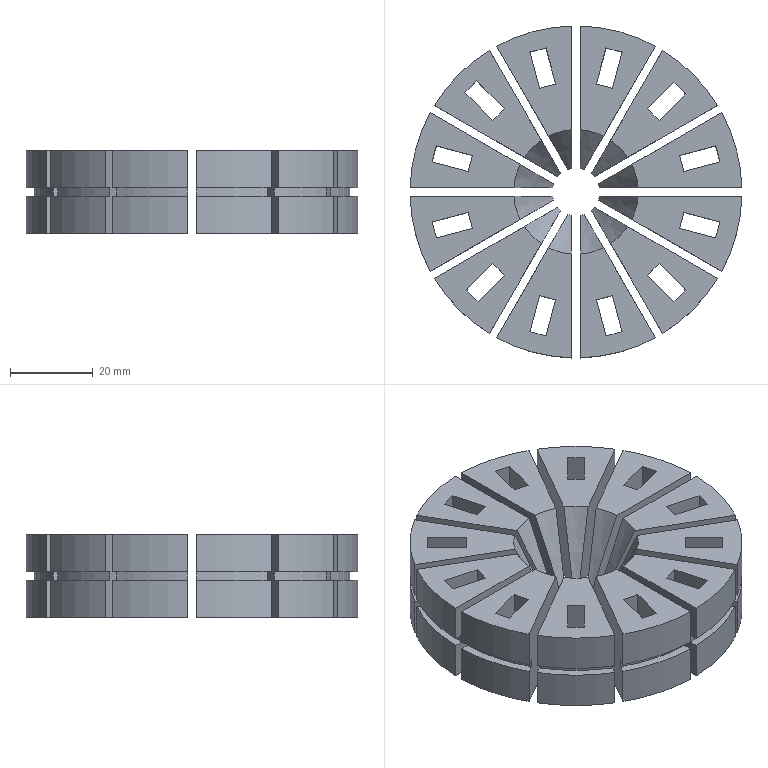Part | NX | features SUBTRACT 12, DATUM_CSYS 4, SKETCH 3, EXTRUDE 2, OFFSET_REGION 1, SWP104 1 | 12 solids | 168 faces | box 79.975 x 79.975 x 19.9 mm | volume 69186 mm3 | plane 120 | cylinder 36 | cone 12 | commonest cylinder face diameters 80 x24 76 x12